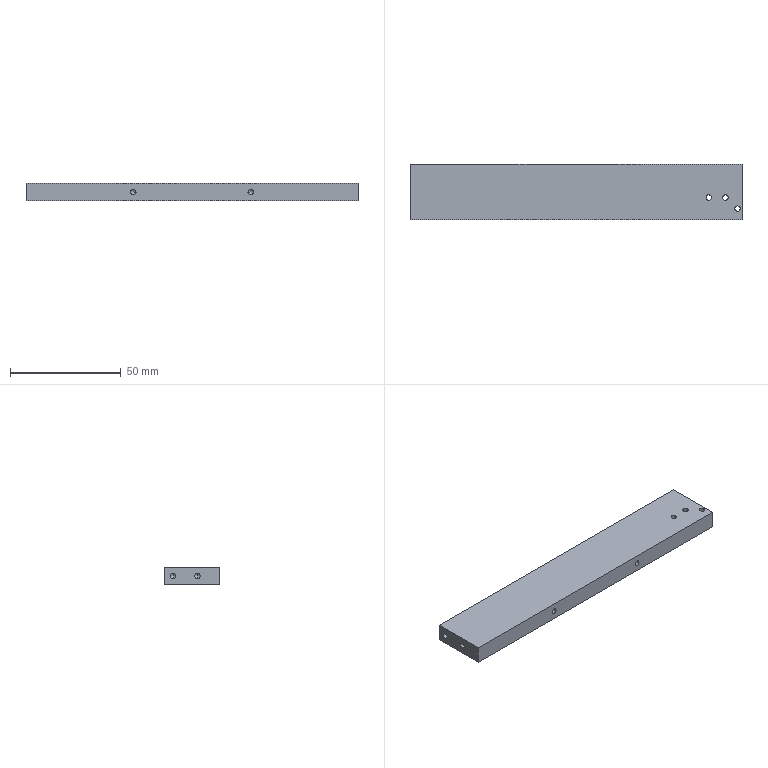Part | SolidWorks | features BaseBody 1 | 1 solid | 40 faces | box 150 x 25 x 8 mm | volume 29604 mm3 | cylinder 22 | cone 12 | plane 6 | commonest cylinder face diameters 2.459 x22
STEP:
#1=CARTESIAN_POINT('',(104.096,10.,0.));
#2=VERTEX_POINT('',#1);
#3=CARTESIAN_POINT('',(101.637,10.,0.));
#4=VERTEX_POINT('',#3);
#5=CARTESIAN_POINT('',(102.866,10.,0.));
#6=DIRECTION('',(0.,0.,-1.));
#7=DIRECTION('',(1.,0.,0.));
#8=AXIS2_PLACEMENT_3D('',#5,#6,#7);
#9=CIRCLE('',#8,1.229);
#10=EDGE_CURVE('',#2,#4,#9,.T.);
#11=ORIENTED_EDGE('',*,*,#10,.T.);
#12=CARTESIAN_POINT('',(101.637,10.,2.77));
#13=VERTEX_POINT('',#12);
#14=CARTESIAN_POINT('',(101.637,10.,-150.193));
#15=DIRECTION('',(0.,0.,1.));
#16=VECTOR('',#15,1000.);
#17=LINE('',#14,#16);
#18=EDGE_CURVE('',#4,#13,#17,.T.);
#19=ORIENTED_EDGE('',*,*,#18,.T.);
#20=CARTESIAN_POINT('',(102.866,8.771,4.));
#21=VERTEX_POINT('',#20);
#22=CARTESIAN_POINT('',(102.866,8.771,4.));
#23=CARTESIAN_POINT('',(102.146,8.771,3.28));
#24=CARTESIAN_POINT('',(101.637,9.28,2.771));
#25=CARTESIAN_POINT('',(101.637,10.,2.77));
#26=(BOUNDED_CURVE()B_SPLINE_CURVE(3,(#22,#23,#24,#25),.UNSPECIFIED.,.F.,.T.)B_SPLINE_CURVE_WITH_KNOTS((4,4),(1.571,3.142),.UNSPECIFIED.)CURVE()GEOMETRIC_REPRESENTATION_ITEM()RATIONAL_B_SPLINE_CURVE((1.,0.8047,0.8047,1.))REPRESENTATION_ITEM(''));
#27=EDGE_CURVE('',#21,#13,#26,.T.);
#28=ORIENTED_EDGE('',*,*,#27,.F.);
#29=CARTESIAN_POINT('',(104.096,10.,2.77));
#30=VERTEX_POINT('',#29);
#31=CARTESIAN_POINT('',(104.096,10.,2.77));
#32=CARTESIAN_POINT('',(104.096,9.28,2.771));
#33=CARTESIAN_POINT('',(103.587,8.771,3.28));
#34=CARTESIAN_POINT('',(102.866,8.771,4.));
#35=(BOUNDED_CURVE()B_SPLINE_CURVE(3,(#31,#32,#33,#34),.UNSPECIFIED.,.F.,.T.)B_SPLINE_CURVE_WITH_KNOTS((4,4),(0.,1.571),.UNSPECIFIED.)CURVE()GEOMETRIC_REPRESENTATION_ITEM()RATIONAL_B_SPLINE_CURVE((1.,0.8047,0.8047,1.))REPRESENTATION_ITEM(''));
#36=EDGE_CURVE('',#30,#21,#35,.T.);
#37=ORIENTED_EDGE('',*,*,#36,.F.);
#38=CARTESIAN_POINT('',(104.096,10.,-150.193));
#39=DIRECTION('',(0.,0.,1.));
#40=VECTOR('',#39,1000.);
#41=LINE('',#38,#40);
#42=EDGE_CURVE('',#2,#30,#41,.T.);
#43=ORIENTED_EDGE('',*,*,#42,.F.);
#44=EDGE_LOOP('',(#11,#19,#28,#37,#43));
#45=FACE_OUTER_BOUND('',#44,.T.);
#46=CARTESIAN_POINT('',(102.866,10.,-150.193));
#47=DIRECTION('',(0.,0.,1.));
#48=DIRECTION('',(1.,0.,0.));
#49=AXIS2_PLACEMENT_3D('',#46,#47,#48);
#50=CYLINDRICAL_SURFACE('',#49,1.229);
#51=ADVANCED_FACE('',(#45),#50,.F.);
#52=CARTESIAN_POINT('',(96.596,10.,0.));
#53=VERTEX_POINT('',#52);
#54=CARTESIAN_POINT('',(94.137,10.,0.));
#55=VERTEX_POINT('',#54);
#56=CARTESIAN_POINT('',(95.366,10.,0.));
#57=DIRECTION('',(0.,0.,-1.));
#58=DIRECTION('',(1.,0.,0.));
#59=AXIS2_PLACEMENT_3D('',#56,#57,#58);
#60=CIRCLE('',#59,1.229);
#61=EDGE_CURVE('',#53,#55,#60,.T.);
#62=ORIENTED_EDGE('',*,*,#61,.T.);
#63=CARTESIAN_POINT('',(94.137,10.,8.));
#64=VERTEX_POINT('',#63);
#65=CARTESIAN_POINT('',(94.137,10.,-150.193));
#66=DIRECTION('',(0.,0.,1.));
#67=VECTOR('',#66,1000.);
#68=LINE('',#65,#67);
#69=EDGE_CURVE('',#55,#64,#68,.T.);
#70=ORIENTED_EDGE('',*,*,#69,.T.);
#71=CARTESIAN_POINT('',(96.596,10.,8.));
#72=VERTEX_POINT('',#71);
#73=CARTESIAN_POINT('',(95.366,10.,8.));
#74=DIRECTION('',(0.,0.,-1.));
#75=DIRECTION('',(1.,0.,0.));
#76=AXIS2_PLACEMENT_3D('',#73,#74,#75);
#77=CIRCLE('',#76,1.229);
#78=EDGE_CURVE('',#72,#64,#77,.T.);
#79=ORIENTED_EDGE('',*,*,#78,.F.);
#80=CARTESIAN_POINT('',(96.596,10.,-150.193));
#81=DIRECTION('',(0.,0.,1.));
#82=VECTOR('',#81,1000.);
#83=LINE('',#80,#82);
#84=EDGE_CURVE('',#53,#72,#83,.T.);
#85=ORIENTED_EDGE('',*,*,#84,.F.);
#86=EDGE_LOOP('',(#62,#70,#79,#85));
#87=FACE_OUTER_BOUND('',#86,.T.);
#88=CARTESIAN_POINT('',(95.366,10.,-150.193));
#89=DIRECTION('',(0.,0.,1.));
#90=DIRECTION('',(1.,0.,0.));
#91=AXIS2_PLACEMENT_3D('',#88,#89,#90);
#92=CYLINDRICAL_SURFACE('',#91,1.229);
#93=ADVANCED_FACE('',(#87),#92,.F.);
#94=CARTESIAN_POINT('',(109.596,5.,0.));
#95=VERTEX_POINT('',#94);
#96=CARTESIAN_POINT('',(107.137,5.,0.));
#97=VERTEX_POINT('',#96);
#98=CARTESIAN_POINT('',(108.366,5.,0.));
#99=DIRECTION('',(0.,0.,-1.));
#100=DIRECTION('',(1.,0.,0.));
#101=AXIS2_PLACEMENT_3D('',#98,#99,#100);
#102=CIRCLE('',#101,1.229);
#103=EDGE_CURVE('',#95,#97,#102,.T.);
#104=ORIENTED_EDGE('',*,*,#103,.T.);
#105=CARTESIAN_POINT('',(107.137,5.,8.));
#106=VERTEX_POINT('',#105);
#107=CARTESIAN_POINT('',(107.137,5.,-150.193));
#108=DIRECTION('',(0.,0.,1.));
#109=VECTOR('',#108,1000.);
#110=LINE('',#107,#109);
#111=EDGE_CURVE('',#97,#106,#110,.T.);
#112=ORIENTED_EDGE('',*,*,#111,.T.);
#113=CARTESIAN_POINT('',(109.596,5.,8.));
#114=VERTEX_POINT('',#113);
#115=CARTESIAN_POINT('',(108.366,5.,8.));
#116=DIRECTION('',(0.,0.,-1.));
#117=DIRECTION('',(1.,0.,0.));
#118=AXIS2_PLACEMENT_3D('',#115,#116,#117);
#119=CIRCLE('',#118,1.229);
#120=EDGE_CURVE('',#114,#106,#119,.T.);
#121=ORIENTED_EDGE('',*,*,#120,.F.);
#122=CARTESIAN_POINT('',(109.596,5.,-150.193));
#123=DIRECTION('',(0.,0.,1.));
#124=VECTOR('',#123,1000.);
#125=LINE('',#122,#124);
#126=EDGE_CURVE('',#95,#114,#125,.T.);
#127=ORIENTED_EDGE('',*,*,#126,.F.);
#128=EDGE_LOOP('',(#104,#112,#121,#127));
#129=FACE_OUTER_BOUND('',#128,.T.);
#130=CARTESIAN_POINT('',(108.366,5.,-150.193));
#131=DIRECTION('',(0.,0.,1.));
#132=DIRECTION('',(1.,0.,0.));
#133=AXIS2_PLACEMENT_3D('',#130,#131,#132);
#134=CYLINDRICAL_SURFACE('',#133,1.229);
#135=ADVANCED_FACE('',(#129),#134,.F.);
#136=CARTESIAN_POINT('',(100.366,10.,5.229));
#137=VERTEX_POINT('',#136);
#138=CARTESIAN_POINT('',(100.366,10.,2.771));
#139=VERTEX_POINT('',#138);
#140=CARTESIAN_POINT('',(100.366,10.,4.));
#141=DIRECTION('',(1.,0.,0.));
#142=DIRECTION('',(0.,0.,-1.));
#143=AXIS2_PLACEMENT_3D('',#140,#141,#142);
#144=CIRCLE('',#143,1.23);
#145=EDGE_CURVE('',#137,#139,#144,.T.);
#146=ORIENTED_EDGE('',*,*,#145,.F.);
#147=CARTESIAN_POINT('',(101.637,10.,5.229));
#148=VERTEX_POINT('',#147);
#149=CARTESIAN_POINT('',(105.366,10.,5.229));
#150=DIRECTION('',(1.,0.,0.));
#151=VECTOR('',#150,1000.);
#152=LINE('',#149,#151);
#153=EDGE_CURVE('',#137,#148,#152,.T.);
#154=ORIENTED_EDGE('',*,*,#153,.T.);
#155=CARTESIAN_POINT('',(102.866,8.771,4.));
#156=CARTESIAN_POINT('',(102.146,8.771,4.72));
#157=CARTESIAN_POINT('',(101.637,9.28,5.23));
#158=CARTESIAN_POINT('',(101.637,10.,5.229));
#159=(BOUNDED_CURVE()B_SPLINE_CURVE(3,(#155,#156,#157,#158),.UNSPECIFIED.,.F.,.T.)B_SPLINE_CURVE_WITH_KNOTS((4,4),(4.712,6.283),.UNSPECIFIED.)CURVE()GEOMETRIC_REPRESENTATION_ITEM()RATIONAL_B_SPLINE_CURVE((1.,0.8047,0.8047,1.))REPRESENTATION_ITEM(''));
#160=EDGE_CURVE('',#21,#148,#159,.T.);
#161=ORIENTED_EDGE('',*,*,#160,.F.);
#162=ORIENTED_EDGE('',*,*,#27,.T.);
#163=CARTESIAN_POINT('',(105.366,10.,2.77));
#164=DIRECTION('',(1.,0.,0.));
#165=VECTOR('',#164,1000.);
#166=LINE('',#163,#165);
#167=EDGE_CURVE('',#139,#13,#166,.T.);
#168=ORIENTED_EDGE('',*,*,#167,.F.);
#169=EDGE_LOOP('',(#146,#154,#161,#162,#168));
#170=FACE_OUTER_BOUND('',#169,.T.);
#171=CARTESIAN_POINT('',(105.366,10.,4.));
#172=DIRECTION('',(1.,0.,0.));
#173=DIRECTION('',(0.,0.,-1.));
#174=AXIS2_PLACEMENT_3D('',#171,#172,#173);
#175=CYLINDRICAL_SURFACE('',#174,1.23);
#176=ADVANCED_FACE('',(#170),#175,.F.);
#177=CARTESIAN_POINT('',(104.096,10.,5.229));
#178=VERTEX_POINT('',#177);
#179=CARTESIAN_POINT('',(104.096,10.,5.229));
#180=CARTESIAN_POINT('',(104.096,9.28,5.23));
#181=CARTESIAN_POINT('',(103.587,8.771,4.72));
#182=CARTESIAN_POINT('',(102.866,8.771,4.));
#183=(BOUNDED_CURVE()B_SPLINE_CURVE(3,(#179,#180,#181,#182),.UNSPECIFIED.,.F.,.F.)B_SPLINE_CURVE_WITH_KNOTS((4,4),(0.,1.571),.UNSPECIFIED.)CURVE()GEOMETRIC_REPRESENTATION_ITEM()RATIONAL_B_SPLINE_CURVE((1.,0.8047,0.8047,1.))REPRESENTATION_ITEM(''));
#184=EDGE_CURVE('',#178,#21,#183,.T.);
#185=ORIENTED_EDGE('',*,*,#184,.F.);
#186=CARTESIAN_POINT('',(110.366,10.,5.23));
#187=VERTEX_POINT('',#186);
#188=CARTESIAN_POINT('',(105.366,10.,5.229));
#189=DIRECTION('',(1.,0.,0.));
#190=VECTOR('',#189,1000.);
#191=LINE('',#188,#190);
#192=EDGE_CURVE('',#178,#187,#191,.T.);
#193=ORIENTED_EDGE('',*,*,#192,.T.);
#194=CARTESIAN_POINT('',(110.366,10.,2.77));
#195=VERTEX_POINT('',#194);
#196=CARTESIAN_POINT('',(110.366,10.,4.));
#197=DIRECTION('',(-1.,0.,0.));
#198=DIRECTION('',(0.,0.,-1.));
#199=AXIS2_PLACEMENT_3D('',#196,#197,#198);
#200=CIRCLE('',#199,1.23);
#201=EDGE_CURVE('',#195,#187,#200,.T.);
#202=ORIENTED_EDGE('',*,*,#201,.F.);
#203=CARTESIAN_POINT('',(105.366,10.,2.77));
#204=DIRECTION('',(1.,0.,0.));
#205=VECTOR('',#204,1000.);
#206=LINE('',#203,#205);
#207=EDGE_CURVE('',#30,#195,#206,.T.);
#208=ORIENTED_EDGE('',*,*,#207,.F.);
#209=ORIENTED_EDGE('',*,*,#36,.T.);
#210=EDGE_LOOP('',(#185,#193,#202,#208,#209));
#211=FACE_OUTER_BOUND('',#210,.T.);
#212=CARTESIAN_POINT('',(105.366,10.,4.));
#213=DIRECTION('',(1.,0.,0.));
#214=DIRECTION('',(0.,0.,-1.));
#215=AXIS2_PLACEMENT_3D('',#212,#213,#214);
#216=CYLINDRICAL_SURFACE('',#215,1.23);
#217=ADVANCED_FACE('',(#211),#216,.F.);
#218=CARTESIAN_POINT('',(100.366,21.,5.229));
#219=VERTEX_POINT('',#218);
#220=CARTESIAN_POINT('',(100.366,21.,2.771));
#221=VERTEX_POINT('',#220);
#222=CARTESIAN_POINT('',(100.366,21.,4.));
#223=DIRECTION('',(1.,0.,0.));
#224=DIRECTION('',(0.,0.,-1.));
#225=AXIS2_PLACEMENT_3D('',#222,#223,#224);
#226=CIRCLE('',#225,1.23);
#227=EDGE_CURVE('',#219,#221,#226,.T.);
#228=ORIENTED_EDGE('',*,*,#227,.F.);
#229=CARTESIAN_POINT('',(110.366,21.,5.23));
#230=VERTEX_POINT('',#229);
#231=CARTESIAN_POINT('',(105.366,21.,5.229));
#232=DIRECTION('',(1.,0.,0.));
#233=VECTOR('',#232,1000.);
#234=LINE('',#231,#233);
#235=EDGE_CURVE('',#219,#230,#234,.T.);
#236=ORIENTED_EDGE('',*,*,#235,.T.);
#237=CARTESIAN_POINT('',(110.366,21.,2.77));
#238=VERTEX_POINT('',#237);
#239=CARTESIAN_POINT('',(110.366,21.,4.));
#240=DIRECTION('',(-1.,0.,0.));
#241=DIRECTION('',(0.,0.,-1.));
#242=AXIS2_PLACEMENT_3D('',#239,#240,#241);
#243=CIRCLE('',#242,1.23);
#244=EDGE_CURVE('',#238,#230,#243,.T.);
#245=ORIENTED_EDGE('',*,*,#244,.F.);
#246=CARTESIAN_POINT('',(105.366,21.,2.77));
#247=DIRECTION('',(1.,0.,0.));
#248=VECTOR('',#247,1000.);
#249=LINE('',#246,#248);
#250=EDGE_CURVE('',#221,#238,#249,.T.);
#251=ORIENTED_EDGE('',*,*,#250,.F.);
#252=EDGE_LOOP('',(#228,#236,#245,#251));
#253=FACE_OUTER_BOUND('',#252,.T.);
#254=CARTESIAN_POINT('',(105.366,21.,4.));
#255=DIRECTION('',(1.,0.,0.));
#256=DIRECTION('',(0.,0.,-1.));
#257=AXIS2_PLACEMENT_3D('',#254,#255,#256);
#258=CYLINDRICAL_SURFACE('',#257,1.23);
#259=ADVANCED_FACE('',(#253),#258,.F.);
#260=CARTESIAN_POINT('',(60.637,10.,4.));
#261=VERTEX_POINT('',#260);
#262=CARTESIAN_POINT('',(63.096,10.,4.));
#263=VERTEX_POINT('',#262);
#264=CARTESIAN_POINT('',(61.866,10.,4.));
#265=DIRECTION('',(0.,-1.,0.));
#266=DIRECTION('',(1.,0.,0.));
#267=AXIS2_PLACEMENT_3D('',#264,#265,#266);
#268=CIRCLE('',#267,1.23);
#269=EDGE_CURVE('',#261,#263,#268,.T.);
#270=ORIENTED_EDGE('',*,*,#269,.F.);
#271=CARTESIAN_POINT('',(60.637,0.,4.));
#272=VERTEX_POINT('',#271);
#273=CARTESIAN_POINT('',(60.637,5.,4.));
#274=DIRECTION('',(0.,-1.,0.));
#275=VECTOR('',#274,1000.);
#276=LINE('',#273,#275);
#277=EDGE_CURVE('',#261,#272,#276,.T.);
#278=ORIENTED_EDGE('',*,*,#277,.T.);
#279=CARTESIAN_POINT('',(63.096,0.,4.));
#280=VERTEX_POINT('',#279);
#281=CARTESIAN_POINT('',(61.866,0.,4.));
#282=DIRECTION('',(0.,1.,0.));
#283=DIRECTION('',(1.,0.,0.));
#284=AXIS2_PLACEMENT_3D('',#281,#282,#283);
#285=CIRCLE('',#284,1.23);
#286=EDGE_CURVE('',#280,#272,#285,.T.);
#287=ORIENTED_EDGE('',*,*,#286,.F.);
#288=CARTESIAN_POINT('',(63.096,5.,4.));
#289=DIRECTION('',(0.,-1.,0.));
#290=VECTOR('',#289,1000.);
#291=LINE('',#288,#290);
#292=EDGE_CURVE('',#263,#280,#291,.T.);
#293=ORIENTED_EDGE('',*,*,#292,.F.);
#294=EDGE_LOOP('',(#270,#278,#287,#293));
#295=FACE_OUTER_BOUND('',#294,.T.);
#296=CARTESIAN_POINT('',(61.866,5.,4.));
#297=DIRECTION('',(0.,-1.,0.));
#298=DIRECTION('',(1.,0.,0.));
#299=AXIS2_PLACEMENT_3D('',#296,#297,#298);
#300=CYLINDRICAL_SURFACE('',#299,1.23);
#301=ADVANCED_FACE('',(#295),#300,.F.);
#302=CARTESIAN_POINT('',(7.637,10.,4.));
#303=VERTEX_POINT('',#302);
#304=CARTESIAN_POINT('',(10.096,10.,4.));
#305=VERTEX_POINT('',#304);
#306=CARTESIAN_POINT('',(8.866,10.,4.));
#307=DIRECTION('',(0.,-1.,0.));
#308=DIRECTION('',(1.,0.,0.));
#309=AXIS2_PLACEMENT_3D('',#306,#307,#308);
#310=CIRCLE('',#309,1.229);
#311=EDGE_CURVE('',#303,#305,#310,.T.);
#312=ORIENTED_EDGE('',*,*,#311,.F.);
#313=CARTESIAN_POINT('',(7.637,0.,4.));
#314=VERTEX_POINT('',#313);
#315=CARTESIAN_POINT('',(7.637,5.,4.));
#316=DIRECTION('',(0.,-1.,0.));
#317=VECTOR('',#316,1000.);
#318=LINE('',#315,#317);
#319=EDGE_CURVE('',#303,#314,#318,.T.);
#320=ORIENTED_EDGE('',*,*,#319,.T.);
#321=CARTESIAN_POINT('',(10.096,0.,4.));
#322=VERTEX_POINT('',#321);
#323=CARTESIAN_POINT('',(8.866,0.,4.));
#324=DIRECTION('',(0.,1.,0.));
#325=DIRECTION('',(1.,0.,0.));
#326=AXIS2_PLACEMENT_3D('',#323,#324,#325);
#327=CIRCLE('',#326,1.229);
#328=EDGE_CURVE('',#322,#314,#327,.T.);
#329=ORIENTED_EDGE('',*,*,#328,.F.);
#330=CARTESIAN_POINT('',(10.096,5.,4.));
#331=DIRECTION('',(0.,-1.,0.));
#332=VECTOR('',#331,1000.);
#333=LINE('',#330,#332);
#334=EDGE_CURVE('',#305,#322,#333,.T.);
#335=ORIENTED_EDGE('',*,*,#334,.F.);
#336=EDGE_LOOP('',(#312,#320,#329,#335));
#337=FACE_OUTER_BOUND('',#336,.T.);
#338=CARTESIAN_POINT('',(8.866,5.,4.));
#339=DIRECTION('',(0.,-1.,0.));
#340=DIRECTION('',(1.,0.,0.));
#341=AXIS2_PLACEMENT_3D('',#338,#339,#340);
#342=CYLINDRICAL_SURFACE('',#341,1.229);
#343=ADVANCED_FACE('',(#337),#342,.F.);
#344=CARTESIAN_POINT('',(-29.634,10.,2.771));
#345=VERTEX_POINT('',#344);
#346=CARTESIAN_POINT('',(-29.634,10.,5.229));
#347=VERTEX_POINT('',#346);
#348=CARTESIAN_POINT('',(-29.634,10.,4.));
#349=DIRECTION('',(-1.,0.,0.));
#350=DIRECTION('',(0.,0.,1.));
#351=AXIS2_PLACEMENT_3D('',#348,#349,#350);
#352=CIRCLE('',#351,1.229);
#353=EDGE_CURVE('',#345,#347,#352,.T.);
#354=ORIENTED_EDGE('',*,*,#353,.F.);
#355=CARTESIAN_POINT('',(-39.634,10.,2.77));
#356=VERTEX_POINT('',#355);
#357=CARTESIAN_POINT('',(-34.634,10.,2.77));
#358=DIRECTION('',(-1.,0.,0.));
#359=VECTOR('',#358,1000.);
#360=LINE('',#357,#359);
#361=EDGE_CURVE('',#345,#356,#360,.T.);
#362=ORIENTED_EDGE('',*,*,#361,.T.);
#363=CARTESIAN_POINT('',(-39.634,10.,5.229));
#364=VERTEX_POINT('',#363);
#365=CARTESIAN_POINT('',(-39.634,10.,4.));
#366=DIRECTION('',(1.,0.,0.));
#367=DIRECTION('',(0.,0.,1.));
#368=AXIS2_PLACEMENT_3D('',#365,#366,#367);
#369=CIRCLE('',#368,1.229);
#370=EDGE_CURVE('',#364,#356,#369,.T.);
#371=ORIENTED_EDGE('',*,*,#370,.F.);
#372=CARTESIAN_POINT('',(-34.634,10.,5.229));
#373=DIRECTION('',(-1.,0.,0.));
#374=VECTOR('',#373,1000.);
#375=LINE('',#372,#374);
#376=EDGE_CURVE('',#347,#364,#375,.T.);
#377=ORIENTED_EDGE('',*,*,#376,.F.);
#378=EDGE_LOOP('',(#354,#362,#371,#377));
#379=FACE_OUTER_BOUND('',#378,.T.);
#380=CARTESIAN_POINT('',(-34.634,10.,4.));
#381=DIRECTION('',(-1.,0.,0.));
#382=DIRECTION('',(0.,0.,1.));
#383=AXIS2_PLACEMENT_3D('',#380,#381,#382);
#384=CYLINDRICAL_SURFACE('',#383,1.229);
#385=ADVANCED_FACE('',(#379),#384,.F.);
#386=CARTESIAN_POINT('',(-29.634,21.,2.771));
#387=VERTEX_POINT('',#386);
#388=CARTESIAN_POINT('',(-29.634,21.,5.229));
#389=VERTEX_POINT('',#388);
#390=CARTESIAN_POINT('',(-29.634,21.,4.));
#391=DIRECTION('',(-1.,0.,0.));
#392=DIRECTION('',(0.,0.,1.));
#393=AXIS2_PLACEMENT_3D('',#390,#391,#392);
#394=CIRCLE('',#393,1.229);
#395=EDGE_CURVE('',#387,#389,#394,.T.);
#396=ORIENTED_EDGE('',*,*,#395,.F.);
#397=CARTESIAN_POINT('',(-39.634,21.,2.77));
#398=VERTEX_POINT('',#397);
#399=CARTESIAN_POINT('',(-34.634,21.,2.77));
#400=DIRECTION('',(-1.,0.,0.));
#401=VECTOR('',#400,1000.);
#402=LINE('',#399,#401);
#403=EDGE_CURVE('',#387,#398,#402,.T.);
#404=ORIENTED_EDGE('',*,*,#403,.T.);
#405=CARTESIAN_POINT('',(-39.634,21.,5.229));
#406=VERTEX_POINT('',#405);
#407=CARTESIAN_POINT('',(-39.634,21.,4.));
#408=DIRECTION('',(1.,0.,0.));
#409=DIRECTION('',(0.,0.,1.));
#410=AXIS2_PLACEMENT_3D('',#407,#408,#409);
#411=CIRCLE('',#410,1.229);
#412=EDGE_CURVE('',#406,#398,#411,.T.);
#413=ORIENTED_EDGE('',*,*,#412,.F.);
#414=CARTESIAN_POINT('',(-34.634,21.,5.229));
#415=DIRECTION('',(-1.,0.,0.));
#416=VECTOR('',#415,1000.);
#417=LINE('',#414,#416);
#418=EDGE_CURVE('',#389,#406,#417,.T.);
#419=ORIENTED_EDGE('',*,*,#418,.F.);
#420=EDGE_LOOP('',(#396,#404,#413,#419));
#421=FACE_OUTER_BOUND('',#420,.T.);
#422=CARTESIAN_POINT('',(-34.634,21.,4.));
#423=DIRECTION('',(-1.,0.,0.));
#424=DIRECTION('',(0.,0.,1.));
#425=AXIS2_PLACEMENT_3D('',#422,#423,#424);
#426=CYLINDRICAL_SURFACE('',#425,1.229);
#427=ADVANCED_FACE('',(#421),#426,.F.);
#428=CARTESIAN_POINT('',(99.628,10.,4.));
#429=VERTEX_POINT('',#428);
#430=CARTESIAN_POINT('',(100.366,10.,2.771));
#431=DIRECTION('',(0.515,0.,-0.8572));
#432=VECTOR('',#431,1000.);
#433=LINE('',#430,#432);
#434=EDGE_CURVE('',#429,#139,#433,.T.);
#435=ORIENTED_EDGE('',*,*,#434,.F.);
#436=CARTESIAN_POINT('',(100.366,10.,5.229));
#437=DIRECTION('',(0.515,0.,0.8572));
#438=VECTOR('',#437,1000.);
#439=LINE('',#436,#438);
#440=EDGE_CURVE('',#429,#137,#439,.T.);
#441=ORIENTED_EDGE('',*,*,#440,.T.);
#442=ORIENTED_EDGE('',*,*,#145,.T.);
#443=EDGE_LOOP('',(#435,#441,#442));
#444=FACE_OUTER_BOUND('',#443,.T.);
#445=CARTESIAN_POINT('',(100.366,10.,4.));
#446=DIRECTION('',(1.,0.,0.));
#447=DIRECTION('',(0.,0.,-1.));
#448=AXIS2_PLACEMENT_3D('',#445,#446,#447);
#449=CONICAL_SURFACE('',#448,1.229,1.03);
#450=ADVANCED_FACE('',(#444),#449,.F.);
#451=ORIENTED_EDGE('',*,*,#160,.T.);
#452=CARTESIAN_POINT('',(101.637,10.,8.));
#453=VERTEX_POINT('',#452);
#454=CARTESIAN_POINT('',(101.637,10.,-150.193));
#455=DIRECTION('',(0.,0.,1.));
#456=VECTOR('',#455,1000.);
#457=LINE('',#454,#456);
#458=EDGE_CURVE('',#148,#453,#457,.T.);
#459=ORIENTED_EDGE('',*,*,#458,.T.);
#460=CARTESIAN_POINT('',(104.096,10.,8.));
#461=VERTEX_POINT('',#460);
#462=CARTESIAN_POINT('',(102.866,10.,8.));
#463=DIRECTION('',(0.,0.,-1.));
#464=DIRECTION('',(1.,0.,0.));
#465=AXIS2_PLACEMENT_3D('',#462,#463,#464);
#466=CIRCLE('',#465,1.229);
#467=EDGE_CURVE('',#461,#453,#466,.T.);
#468=ORIENTED_EDGE('',*,*,#467,.F.);
#469=CARTESIAN_POINT('',(104.096,10.,-150.193));
#470=DIRECTION('',(0.,0.,1.));
#471=VECTOR('',#470,1000.);
#472=LINE('',#469,#471);
#473=EDGE_CURVE('',#178,#461,#472,.T.);
#474=ORIENTED_EDGE('',*,*,#473,.F.);
#475=ORIENTED_EDGE('',*,*,#184,.T.);
#476=EDGE_LOOP('',(#451,#459,#468,#474,#475));
#477=FACE_OUTER_BOUND('',#476,.T.);
#478=CARTESIAN_POINT('',(102.866,10.,-150.193));
#479=DIRECTION('',(0.,0.,1.));
#480=DIRECTION('',(1.,0.,0.));
#481=AXIS2_PLACEMENT_3D('',#478,#479,#480);
#482=CYLINDRICAL_SURFACE('',#481,1.229);
#483=ADVANCED_FACE('',(#477),#482,.F.);
#484=CARTESIAN_POINT('',(99.628,21.,4.));
#485=VERTEX_POINT('',#484);
#486=CARTESIAN_POINT('',(100.366,21.,2.771));
#487=DIRECTION('',(0.515,0.,-0.8572));
#488=VECTOR('',#487,1000.);
#489=LINE('',#486,#488);
#490=EDGE_CURVE('',#485,#221,#489,.T.);
#491=ORIENTED_EDGE('',*,*,#490,.F.);
#492=CARTESIAN_POINT('',(100.366,21.,5.229));
#493=DIRECTION('',(0.515,0.,0.8572));
#494=VECTOR('',#493,1000.);
#495=LINE('',#492,#494);
#496=EDGE_CURVE('',#485,#219,#495,.T.);
#497=ORIENTED_EDGE('',*,*,#496,.T.);
#498=ORIENTED_EDGE('',*,*,#227,.T.);
#499=EDGE_LOOP('',(#491,#497,#498));
#500=FACE_OUTER_BOUND('',#499,.T.);
#501=CARTESIAN_POINT('',(100.366,21.,4.));
#502=DIRECTION('',(1.,0.,0.));
#503=DIRECTION('',(0.,0.,-1.));
#504=AXIS2_PLACEMENT_3D('',#501,#502,#503);
#505=CONICAL_SURFACE('',#504,1.229,1.03);
#506=ADVANCED_FACE('',(#500),#505,.F.);
#507=CARTESIAN_POINT('',(61.866,10.739,4.));
#508=VERTEX_POINT('',#507);
#509=CARTESIAN_POINT('',(63.096,10.,4.));
#510=DIRECTION('',(0.8572,-0.515,0.));
#511=VECTOR('',#510,1000.);
#512=LINE('',#509,#511);
#513=EDGE_CURVE('',#508,#263,#512,.T.);
#514=ORIENTED_EDGE('',*,*,#513,.F.);
#515=CARTESIAN_POINT('',(60.637,10.,4.));
#516=DIRECTION('',(-0.8572,-0.515,0.));
#517=VECTOR('',#516,1000.);
#518=LINE('',#515,#517);
#519=EDGE_CURVE('',#508,#261,#518,.T.);
#520=ORIENTED_EDGE('',*,*,#519,.T.);
#521=ORIENTED_EDGE('',*,*,#269,.T.);
#522=EDGE_LOOP('',(#514,#520,#521));
#523=FACE_OUTER_BOUND('',#522,.T.);
#524=CARTESIAN_POINT('',(61.866,10.,4.));
#525=DIRECTION('',(0.,-1.,0.));
#526=DIRECTION('',(1.,0.,0.));
#527=AXIS2_PLACEMENT_3D('',#524,#525,#526);
#528=CONICAL_SURFACE('',#527,1.229,1.03);
#529=ADVANCED_FACE('',(#523),#528,.F.);
#530=CARTESIAN_POINT('',(8.866,10.739,4.));
#531=VERTEX_POINT('',#530);
#532=CARTESIAN_POINT('',(10.096,10.,4.));
#533=DIRECTION('',(0.8572,-0.515,0.));
#534=VECTOR('',#533,1000.);
#535=LINE('',#532,#534);
#536=EDGE_CURVE('',#531,#305,#535,.T.);
#537=ORIENTED_EDGE('',*,*,#536,.F.);
#538=CARTESIAN_POINT('',(7.637,10.,4.));
#539=DIRECTION('',(-0.8572,-0.515,0.));
#540=VECTOR('',#539,1000.);
#541=LINE('',#538,#540);
#542=EDGE_CURVE('',#531,#303,#541,.T.);
#543=ORIENTED_EDGE('',*,*,#542,.T.);
#544=ORIENTED_EDGE('',*,*,#311,.T.);
#545=EDGE_LOOP('',(#537,#543,#544));
#546=FACE_OUTER_BOUND('',#545,.T.);
#547=CARTESIAN_POINT('',(8.866,10.,4.));
#548=DIRECTION('',(0.,-1.,0.));
#549=DIRECTION('',(1.,0.,0.));
#550=AXIS2_PLACEMENT_3D('',#547,#548,#549);
#551=CONICAL_SURFACE('',#550,1.229,1.03);
#552=ADVANCED_FACE('',(#546),#551,.F.);
#553=CARTESIAN_POINT('',(-28.895,10.,4.));
#554=VERTEX_POINT('',#553);
#555=CARTESIAN_POINT('',(-29.634,10.,5.229));
#556=DIRECTION('',(-0.515,0.,0.8572));
#557=VECTOR('',#556,1000.);
#558=LINE('',#555,#557);
#559=EDGE_CURVE('',#554,#347,#558,.T.);
#560=ORIENTED_EDGE('',*,*,#559,.F.);
#561=CARTESIAN_POINT('',(-29.634,10.,2.771));
#562=DIRECTION('',(-0.515,0.,-0.8572));
#563=VECTOR('',#562,1000.);
#564=LINE('',#561,#563);
#565=EDGE_CURVE('',#554,#345,#564,.T.);
#566=ORIENTED_EDGE('',*,*,#565,.T.);
#567=ORIENTED_EDGE('',*,*,#353,.T.);
#568=EDGE_LOOP('',(#560,#566,#567));
#569=FACE_OUTER_BOUND('',#568,.T.);
#570=CARTESIAN_POINT('',(-29.634,10.,4.));
#571=DIRECTION('',(-1.,0.,0.));
#572=DIRECTION('',(0.,0.,1.));
#573=AXIS2_PLACEMENT_3D('',#570,#571,#572);
#574=CONICAL_SURFACE('',#573,1.229,1.03);
#575=ADVANCED_FACE('',(#569),#574,.F.);
#576=CARTESIAN_POINT('',(-28.895,21.,4.));
#577=VERTEX_POINT('',#576);
#578=CARTESIAN_POINT('',(-29.634,21.,5.229));
#579=DIRECTION('',(-0.515,0.,0.8572));
#580=VECTOR('',#579,1000.);
#581=LINE('',#578,#580);
#582=EDGE_CURVE('',#577,#389,#581,.T.);
#583=ORIENTED_EDGE('',*,*,#582,.F.);
#584=CARTESIAN_POINT('',(-29.634,21.,2.771));
#585=DIRECTION('',(-0.515,0.,-0.8572));
#586=VECTOR('',#585,1000.);
#587=LINE('',#584,#586);
#588=EDGE_CURVE('',#577,#387,#587,.T.);
#589=ORIENTED_EDGE('',*,*,#588,.T.);
#590=ORIENTED_EDGE('',*,*,#395,.T.);
#591=EDGE_LOOP('',(#583,#589,#590));
#592=FACE_OUTER_BOUND('',#591,.T.);
#593=CARTESIAN_POINT('',(-29.634,21.,4.));
#594=DIRECTION('',(-1.,0.,0.));
#595=DIRECTION('',(0.,0.,1.));
#596=AXIS2_PLACEMENT_3D('',#593,#594,#595);
#597=CONICAL_SURFACE('',#596,1.229,1.03);
#598=ADVANCED_FACE('',(#592),#597,.F.);
#599=ORIENTED_EDGE('',*,*,#10,.F.);
#600=CARTESIAN_POINT('',(102.866,10.,0.));
#601=DIRECTION('',(0.,0.,-1.));
#602=DIRECTION('',(1.,0.,0.));
#603=AXIS2_PLACEMENT_3D('',#600,#601,#602);
#604=CIRCLE('',#603,1.229);
#605=EDGE_CURVE('',#4,#2,#604,.T.);
#606=ORIENTED_EDGE('',*,*,#605,.F.);
#607=EDGE_LOOP('',(#599,#606));
#608=FACE_BOUND('',#607,.T.);
#609=ORIENTED_EDGE('',*,*,#61,.F.);
#610=CARTESIAN_POINT('',(95.366,10.,0.));
#611=DIRECTION('',(0.,0.,-1.));
#612=DIRECTION('',(1.,0.,0.));
#613=AXIS2_PLACEMENT_3D('',#610,#611,#612);
#614=CIRCLE('',#613,1.229);
#615=EDGE_CURVE('',#55,#53,#614,.T.);
#616=ORIENTED_EDGE('',*,*,#615,.F.);
#617=EDGE_LOOP('',(#609,#616));
#618=FACE_BOUND('',#617,.T.);
#619=ORIENTED_EDGE('',*,*,#103,.F.);
#620=CARTESIAN_POINT('',(108.366,5.,0.));
#621=DIRECTION('',(0.,0.,-1.));
#622=DIRECTION('',(1.,0.,0.));
#623=AXIS2_PLACEMENT_3D('',#620,#621,#622);
#624=CIRCLE('',#623,1.229);
#625=EDGE_CURVE('',#97,#95,#624,.T.);
#626=ORIENTED_EDGE('',*,*,#625,.F.);
#627=EDGE_LOOP('',(#619,#626));
#628=FACE_BOUND('',#627,.T.);
#629=CARTESIAN_POINT('',(110.366,0.,0.));
#630=VERTEX_POINT('',#629);
#631=CARTESIAN_POINT('',(110.366,25.,0.));
#632=VERTEX_POINT('',#631);
#633=CARTESIAN_POINT('',(110.366,12.5,0.));
#634=DIRECTION('',(0.,1.,0.));
#635=VECTOR('',#634,1000.);
#636=LINE('',#633,#635);
#637=EDGE_CURVE('',#630,#632,#636,.T.);
#638=ORIENTED_EDGE('',*,*,#637,.F.);
#639=CARTESIAN_POINT('',(-39.634,0.,0.));
#640=VERTEX_POINT('',#639);
#641=CARTESIAN_POINT('',(35.366,0.,0.));
#642=DIRECTION('',(1.,0.,0.));
#643=VECTOR('',#642,1000.);
#644=LINE('',#641,#643);
#645=EDGE_CURVE('',#640,#630,#644,.T.);
#646=ORIENTED_EDGE('',*,*,#645,.F.);
#647=CARTESIAN_POINT('',(-39.634,25.,0.));
#648=VERTEX_POINT('',#647);
#649=CARTESIAN_POINT('',(-39.634,12.5,0.));
#650=DIRECTION('',(0.,-1.,0.));
#651=VECTOR('',#650,1000.);
#652=LINE('',#649,#651);
#653=EDGE_CURVE('',#648,#640,#652,.T.);
#654=ORIENTED_EDGE('',*,*,#653,.F.);
#655=CARTESIAN_POINT('',(35.366,25.,0.));
#656=DIRECTION('',(-1.,0.,0.));
#657=VECTOR('',#656,1000.);
#658=LINE('',#655,#657);
#659=EDGE_CURVE('',#632,#648,#658,.T.);
#660=ORIENTED_EDGE('',*,*,#659,.F.);
#661=EDGE_LOOP('',(#638,#646,#654,#660));
#662=FACE_OUTER_BOUND('',#661,.T.);
#663=CARTESIAN_POINT('',(35.366,12.5,0.));
#664=DIRECTION('',(0.,0.,1.));
#665=DIRECTION('',(1.,0.,0.));
#666=AXIS2_PLACEMENT_3D('',#663,#664,#665);
#667=PLANE('',#666);
#668=ADVANCED_FACE('',(#608,#618,#628,#662),#667,.F.);
#669=ORIENTED_EDGE('',*,*,#18,.F.);
#670=ORIENTED_EDGE('',*,*,#605,.T.);
#671=ORIENTED_EDGE('',*,*,#42,.T.);
#672=CARTESIAN_POINT('',(102.866,11.23,4.));
#673=VERTEX_POINT('',#672);
#674=CARTESIAN_POINT('',(102.866,11.23,4.));
#675=CARTESIAN_POINT('',(103.587,11.23,3.28));
#676=CARTESIAN_POINT('',(104.096,10.72,2.771));
#677=CARTESIAN_POINT('',(104.096,10.,2.77));
#678=(BOUNDED_CURVE()B_SPLINE_CURVE(3,(#674,#675,#676,#677),.UNSPECIFIED.,.F.,.F.)B_SPLINE_CURVE_WITH_KNOTS((4,4),(4.712,6.283),.UNSPECIFIED.)CURVE()GEOMETRIC_REPRESENTATION_ITEM()RATIONAL_B_SPLINE_CURVE((1.,0.8047,0.8047,1.))REPRESENTATION_ITEM(''));
#679=EDGE_CURVE('',#673,#30,#678,.T.);
#680=ORIENTED_EDGE('',*,*,#679,.F.);
#681=CARTESIAN_POINT('',(101.637,10.,2.77));
#682=CARTESIAN_POINT('',(101.637,10.72,2.771));
#683=CARTESIAN_POINT('',(102.146,11.23,3.28));
#684=CARTESIAN_POINT('',(102.866,11.23,4.));
#685=(BOUNDED_CURVE()B_SPLINE_CURVE(3,(#681,#682,#683,#684),.UNSPECIFIED.,.F.,.T.)B_SPLINE_CURVE_WITH_KNOTS((4,4),(3.142,4.712),.UNSPECIFIED.)CURVE()GEOMETRIC_REPRESENTATION_ITEM()RATIONAL_B_SPLINE_CURVE((1.,0.8047,0.8047,1.))REPRESENTATION_ITEM(''));
#686=EDGE_CURVE('',#13,#673,#685,.T.);
#687=ORIENTED_EDGE('',*,*,#686,.F.);
#688=EDGE_LOOP('',(#669,#670,#671,#680,#687));
#689=FACE_OUTER_BOUND('',#688,.T.);
#690=CARTESIAN_POINT('',(102.866,10.,-150.193));
#691=DIRECTION('',(0.,0.,1.));
#692=DIRECTION('',(1.,0.,0.));
#693=AXIS2_PLACEMENT_3D('',#690,#691,#692);
#694=CYLINDRICAL_SURFACE('',#693,1.229);
#695=ADVANCED_FACE('',(#689),#694,.F.);
#696=ORIENTED_EDGE('',*,*,#69,.F.);
#697=ORIENTED_EDGE('',*,*,#615,.T.);
#698=ORIENTED_EDGE('',*,*,#84,.T.);
#699=CARTESIAN_POINT('',(95.366,10.,8.));
#700=DIRECTION('',(0.,0.,-1.));
#701=DIRECTION('',(1.,0.,0.));
#702=AXIS2_PLACEMENT_3D('',#699,#700,#701);
#703=CIRCLE('',#702,1.229);
#704=EDGE_CURVE('',#64,#72,#703,.T.);
#705=ORIENTED_EDGE('',*,*,#704,.F.);
#706=EDGE_LOOP('',(#696,#697,#698,#705));
#707=FACE_OUTER_BOUND('',#706,.T.);
#708=CARTESIAN_POINT('',(95.366,10.,-150.193));
#709=DIRECTION('',(0.,0.,1.));
#710=DIRECTION('',(1.,0.,0.));
#711=AXIS2_PLACEMENT_3D('',#708,#709,#710);
#712=CYLINDRICAL_SURFACE('',#711,1.229);
#713=ADVANCED_FACE('',(#707),#712,.F.);
#714=ORIENTED_EDGE('',*,*,#111,.F.);
#715=ORIENTED_EDGE('',*,*,#625,.T.);
#716=ORIENTED_EDGE('',*,*,#126,.T.);
#717=CARTESIAN_POINT('',(108.366,5.,8.));
#718=DIRECTION('',(0.,0.,-1.));
#719=DIRECTION('',(1.,0.,0.));
#720=AXIS2_PLACEMENT_3D('',#717,#718,#719);
#721=CIRCLE('',#720,1.229);
#722=EDGE_CURVE('',#106,#114,#721,.T.);
#723=ORIENTED_EDGE('',*,*,#722,.F.);
#724=EDGE_LOOP('',(#714,#715,#716,#723));
#725=FACE_OUTER_BOUND('',#724,.T.);
#726=CARTESIAN_POINT('',(108.366,5.,-150.193));
#727=DIRECTION('',(0.,0.,1.));
#728=DIRECTION('',(1.,0.,0.));
#729=AXIS2_PLACEMENT_3D('',#726,#727,#728);
#730=CYLINDRICAL_SURFACE('',#729,1.229);
#731=ADVANCED_FACE('',(#725),#730,.F.);
#732=ORIENTED_EDGE('',*,*,#659,.T.);
#733=CARTESIAN_POINT('',(-39.634,25.,8.));
#734=VERTEX_POINT('',#733);
#735=CARTESIAN_POINT('',(-39.634,25.,0.));
#736=DIRECTION('',(0.,0.,1.));
#737=VECTOR('',#736,1000.);
#738=LINE('',#735,#737);
#739=EDGE_CURVE('',#648,#734,#738,.T.);
#740=ORIENTED_EDGE('',*,*,#739,.T.);
#741=CARTESIAN_POINT('',(110.366,25.,8.));
#742=VERTEX_POINT('',#741);
#743=CARTESIAN_POINT('',(-39.634,25.,8.));
#744=DIRECTION('',(1.,0.,0.));
#745=VECTOR('',#744,1000.);
#746=LINE('',#743,#745);
#747=EDGE_CURVE('',#734,#742,#746,.T.);
#748=ORIENTED_EDGE('',*,*,#747,.T.);
#749=CARTESIAN_POINT('',(110.366,25.,0.));
#750=DIRECTION('',(0.,0.,-1.));
#751=VECTOR('',#750,1000.);
#752=LINE('',#749,#751);
#753=EDGE_CURVE('',#742,#632,#752,.T.);
#754=ORIENTED_EDGE('',*,*,#753,.T.);
#755=EDGE_LOOP('',(#732,#740,#748,#754));
#756=FACE_OUTER_BOUND('',#755,.T.);
#757=CARTESIAN_POINT('',(-39.634,25.,0.));
#758=DIRECTION('',(0.,1.,0.));
#759=DIRECTION('',(0.,0.,1.));
#760=AXIS2_PLACEMENT_3D('',#757,#758,#759);
#761=PLANE('',#760);
#762=ADVANCED_FACE('',(#756),#761,.T.);
#763=ORIENTED_EDGE('',*,*,#201,.T.);
#764=CARTESIAN_POINT('',(110.366,10.,4.));
#765=DIRECTION('',(-1.,0.,0.));
#766=DIRECTION('',(0.,0.,-1.));
#767=AXIS2_PLACEMENT_3D('',#764,#765,#766);
#768=CIRCLE('',#767,1.23);
#769=EDGE_CURVE('',#187,#195,#768,.T.);
#770=ORIENTED_EDGE('',*,*,#769,.T.);
#771=EDGE_LOOP('',(#763,#770));
#772=FACE_BOUND('',#771,.T.);
#773=ORIENTED_EDGE('',*,*,#244,.T.);
#774=CARTESIAN_POINT('',(110.366,21.,4.));
#775=DIRECTION('',(-1.,0.,0.));
#776=DIRECTION('',(0.,0.,-1.));
#777=AXIS2_PLACEMENT_3D('',#774,#775,#776);
#778=CIRCLE('',#777,1.23);
#779=EDGE_CURVE('',#230,#238,#778,.T.);
#780=ORIENTED_EDGE('',*,*,#779,.T.);
#781=EDGE_LOOP('',(#773,#780));
#782=FACE_BOUND('',#781,.T.);
#783=ORIENTED_EDGE('',*,*,#637,.T.);
#784=ORIENTED_EDGE('',*,*,#753,.F.);
#785=CARTESIAN_POINT('',(110.366,0.,8.));
#786=VERTEX_POINT('',#785);
#787=CARTESIAN_POINT('',(110.366,25.,8.));
#788=DIRECTION('',(0.,-1.,0.));
#789=VECTOR('',#788,1000.);
#790=LINE('',#787,#789);
#791=EDGE_CURVE('',#742,#786,#790,.T.);
#792=ORIENTED_EDGE('',*,*,#791,.T.);
#793=CARTESIAN_POINT('',(110.366,0.,0.));
#794=DIRECTION('',(0.,0.,-1.));
#795=VECTOR('',#794,1000.);
#796=LINE('',#793,#795);
#797=EDGE_CURVE('',#786,#630,#796,.T.);
#798=ORIENTED_EDGE('',*,*,#797,.T.);
#799=EDGE_LOOP('',(#783,#784,#792,#798));
#800=FACE_OUTER_BOUND('',#799,.T.);
#801=CARTESIAN_POINT('',(110.366,25.,0.));
#802=DIRECTION('',(1.,0.,0.));
#803=DIRECTION('',(0.,0.,-1.));
#804=AXIS2_PLACEMENT_3D('',#801,#802,#803);
#805=PLANE('',#804);
#806=ADVANCED_FACE('',(#772,#782,#800),#805,.T.);
#807=ORIENTED_EDGE('',*,*,#286,.T.);
#808=CARTESIAN_POINT('',(61.866,0.,4.));
#809=DIRECTION('',(0.,1.,0.));
#810=DIRECTION('',(1.,0.,0.));
#811=AXIS2_PLACEMENT_3D('',#808,#809,#810);
#812=CIRCLE('',#811,1.23);
#813=EDGE_CURVE('',#272,#280,#812,.T.);
#814=ORIENTED_EDGE('',*,*,#813,.T.);
#815=EDGE_LOOP('',(#807,#814));
#816=FACE_BOUND('',#815,.T.);
#817=ORIENTED_EDGE('',*,*,#328,.T.);
#818=CARTESIAN_POINT('',(8.866,0.,4.));
#819=DIRECTION('',(0.,1.,0.));
#820=DIRECTION('',(1.,0.,0.));
#821=AXIS2_PLACEMENT_3D('',#818,#819,#820);
#822=CIRCLE('',#821,1.229);
#823=EDGE_CURVE('',#314,#322,#822,.T.);
#824=ORIENTED_EDGE('',*,*,#823,.T.);
#825=EDGE_LOOP('',(#817,#824));
#826=FACE_BOUND('',#825,.T.);
#827=ORIENTED_EDGE('',*,*,#645,.T.);
#828=ORIENTED_EDGE('',*,*,#797,.F.);
#829=CARTESIAN_POINT('',(-39.634,0.,8.));
#830=VERTEX_POINT('',#829);
#831=CARTESIAN_POINT('',(110.366,0.,8.));
#832=DIRECTION('',(-1.,0.,0.));
#833=VECTOR('',#832,1000.);
#834=LINE('',#831,#833);
#835=EDGE_CURVE('',#786,#830,#834,.T.);
#836=ORIENTED_EDGE('',*,*,#835,.T.);
#837=CARTESIAN_POINT('',(-39.634,0.,0.));
#838=DIRECTION('',(0.,0.,-1.));
#839=VECTOR('',#838,1000.);
#840=LINE('',#837,#839);
#841=EDGE_CURVE('',#830,#640,#840,.T.);
#842=ORIENTED_EDGE('',*,*,#841,.T.);
#843=EDGE_LOOP('',(#827,#828,#836,#842));
#844=FACE_OUTER_BOUND('',#843,.T.);
#845=CARTESIAN_POINT('',(110.366,0.,0.));
#846=DIRECTION('',(0.,-1.,0.));
#847=DIRECTION('',(0.,0.,-1.));
#848=AXIS2_PLACEMENT_3D('',#845,#846,#847);
#849=PLANE('',#848);
#850=ADVANCED_FACE('',(#816,#826,#844),#849,.T.);
#851=ORIENTED_EDGE('',*,*,#370,.T.);
#852=CARTESIAN_POINT('',(-39.634,10.,4.));
#853=DIRECTION('',(1.,0.,0.));
#854=DIRECTION('',(0.,0.,1.));
#855=AXIS2_PLACEMENT_3D('',#852,#853,#854);
#856=CIRCLE('',#855,1.229);
#857=EDGE_CURVE('',#356,#364,#856,.T.);
#858=ORIENTED_EDGE('',*,*,#857,.T.);
#859=EDGE_LOOP('',(#851,#858));
#860=FACE_BOUND('',#859,.T.);
#861=ORIENTED_EDGE('',*,*,#412,.T.);
#862=CARTESIAN_POINT('',(-39.634,21.,4.));
#863=DIRECTION('',(1.,0.,0.));
#864=DIRECTION('',(0.,0.,1.));
#865=AXIS2_PLACEMENT_3D('',#862,#863,#864);
#866=CIRCLE('',#865,1.229);
#867=EDGE_CURVE('',#398,#406,#866,.T.);
#868=ORIENTED_EDGE('',*,*,#867,.T.);
#869=EDGE_LOOP('',(#861,#868));
#870=FACE_BOUND('',#869,.T.);
#871=ORIENTED_EDGE('',*,*,#653,.T.);
#872=ORIENTED_EDGE('',*,*,#841,.F.);
#873=CARTESIAN_POINT('',(-39.634,0.,8.));
#874=DIRECTION('',(0.,1.,0.));
#875=VECTOR('',#874,1000.);
#876=LINE('',#873,#875);
#877=EDGE_CURVE('',#830,#734,#876,.T.);
#878=ORIENTED_EDGE('',*,*,#877,.T.);
#879=ORIENTED_EDGE('',*,*,#739,.F.);
#880=EDGE_LOOP('',(#871,#872,#878,#879));
#881=FACE_OUTER_BOUND('',#880,.T.);
#882=CARTESIAN_POINT('',(-39.634,0.,0.));
#883=DIRECTION('',(-1.,0.,0.));
#884=DIRECTION('',(0.,0.,1.));
#885=AXIS2_PLACEMENT_3D('',#882,#883,#884);
#886=PLANE('',#885);
#887=ADVANCED_FACE('',(#860,#870,#881),#886,.T.);
#888=ORIENTED_EDGE('',*,*,#153,.F.);
#889=CARTESIAN_POINT('',(100.366,10.,4.));
#890=DIRECTION('',(1.,0.,0.));
#891=DIRECTION('',(0.,0.,-1.));
#892=AXIS2_PLACEMENT_3D('',#889,#890,#891);
#893=CIRCLE('',#892,1.23);
#894=EDGE_CURVE('',#139,#137,#893,.T.);
#895=ORIENTED_EDGE('',*,*,#894,.F.);
#896=ORIENTED_EDGE('',*,*,#167,.T.);
#897=ORIENTED_EDGE('',*,*,#686,.T.);
#898=CARTESIAN_POINT('',(101.637,10.,5.229));
#899=CARTESIAN_POINT('',(101.637,10.72,5.23));
#900=CARTESIAN_POINT('',(102.146,11.23,4.72));
#901=CARTESIAN_POINT('',(102.866,11.23,4.));
#902=(BOUNDED_CURVE()B_SPLINE_CURVE(3,(#898,#899,#900,#901),.UNSPECIFIED.,.F.,.T.)B_SPLINE_CURVE_WITH_KNOTS((4,4),(0.,1.571),.UNSPECIFIED.)CURVE()GEOMETRIC_REPRESENTATION_ITEM()RATIONAL_B_SPLINE_CURVE((1.,0.8047,0.8047,1.))REPRESENTATION_ITEM(''));
#903=EDGE_CURVE('',#148,#673,#902,.T.);
#904=ORIENTED_EDGE('',*,*,#903,.F.);
#905=EDGE_LOOP('',(#888,#895,#896,#897,#904));
#906=FACE_OUTER_BOUND('',#905,.T.);
#907=CARTESIAN_POINT('',(105.366,10.,4.));
#908=DIRECTION('',(1.,0.,0.));
#909=DIRECTION('',(0.,0.,-1.));
#910=AXIS2_PLACEMENT_3D('',#907,#908,#909);
#911=CYLINDRICAL_SURFACE('',#910,1.23);
#912=ADVANCED_FACE('',(#906),#911,.F.);
#913=ORIENTED_EDGE('',*,*,#192,.F.);
#914=CARTESIAN_POINT('',(102.866,11.23,4.));
#915=CARTESIAN_POINT('',(103.587,11.23,4.72));
#916=CARTESIAN_POINT('',(104.096,10.72,5.23));
#917=CARTESIAN_POINT('',(104.096,10.,5.229));
#918=(BOUNDED_CURVE()B_SPLINE_CURVE(3,(#914,#915,#916,#917),.UNSPECIFIED.,.F.,.T.)B_SPLINE_CURVE_WITH_KNOTS((4,4),(4.712,6.283),.UNSPECIFIED.)CURVE()GEOMETRIC_REPRESENTATION_ITEM()RATIONAL_B_SPLINE_CURVE((1.,0.8047,0.8047,1.))REPRESENTATION_ITEM(''));
#919=EDGE_CURVE('',#673,#178,#918,.T.);
#920=ORIENTED_EDGE('',*,*,#919,.F.);
#921=ORIENTED_EDGE('',*,*,#679,.T.);
#922=ORIENTED_EDGE('',*,*,#207,.T.);
#923=ORIENTED_EDGE('',*,*,#769,.F.);
#924=EDGE_LOOP('',(#913,#920,#921,#922,#923));
#925=FACE_OUTER_BOUND('',#924,.T.);
#926=CARTESIAN_POINT('',(105.366,10.,4.));
#927=DIRECTION('',(1.,0.,0.));
#928=DIRECTION('',(0.,0.,-1.));
#929=AXIS2_PLACEMENT_3D('',#926,#927,#928);
#930=CYLINDRICAL_SURFACE('',#929,1.23);
#931=ADVANCED_FACE('',(#925),#930,.F.);
#932=ORIENTED_EDGE('',*,*,#467,.T.);
#933=CARTESIAN_POINT('',(102.866,10.,8.));
#934=DIRECTION('',(0.,0.,-1.));
#935=DIRECTION('',(1.,0.,0.));
#936=AXIS2_PLACEMENT_3D('',#933,#934,#935);
#937=CIRCLE('',#936,1.229);
#938=EDGE_CURVE('',#453,#461,#937,.T.);
#939=ORIENTED_EDGE('',*,*,#938,.T.);
#940=EDGE_LOOP('',(#932,#939));
#941=FACE_BOUND('',#940,.T.);
#942=ORIENTED_EDGE('',*,*,#78,.T.);
#943=ORIENTED_EDGE('',*,*,#704,.T.);
#944=EDGE_LOOP('',(#942,#943));
#945=FACE_BOUND('',#944,.T.);
#946=ORIENTED_EDGE('',*,*,#120,.T.);
#947=ORIENTED_EDGE('',*,*,#722,.T.);
#948=EDGE_LOOP('',(#946,#947));
#949=FACE_BOUND('',#948,.T.);
#950=ORIENTED_EDGE('',*,*,#877,.F.);
#951=ORIENTED_EDGE('',*,*,#835,.F.);
#952=ORIENTED_EDGE('',*,*,#791,.F.);
#953=ORIENTED_EDGE('',*,*,#747,.F.);
#954=EDGE_LOOP('',(#950,#951,#952,#953));
#955=FACE_OUTER_BOUND('',#954,.T.);
#956=CARTESIAN_POINT('',(35.366,12.5,8.));
#957=DIRECTION('',(0.,0.,1.));
#958=DIRECTION('',(1.,0.,0.));
#959=AXIS2_PLACEMENT_3D('',#956,#957,#958);
#960=PLANE('',#959);
#961=ADVANCED_FACE('',(#941,#945,#949,#955),#960,.T.);
#962=ORIENTED_EDGE('',*,*,#235,.F.);
#963=CARTESIAN_POINT('',(100.366,21.,4.));
#964=DIRECTION('',(1.,0.,0.));
#965=DIRECTION('',(0.,0.,-1.));
#966=AXIS2_PLACEMENT_3D('',#963,#964,#965);
#967=CIRCLE('',#966,1.23);
#968=EDGE_CURVE('',#221,#219,#967,.T.);
#969=ORIENTED_EDGE('',*,*,#968,.F.);
#970=ORIENTED_EDGE('',*,*,#250,.T.);
#971=ORIENTED_EDGE('',*,*,#779,.F.);
#972=EDGE_LOOP('',(#962,#969,#970,#971));
#973=FACE_OUTER_BOUND('',#972,.T.);
#974=CARTESIAN_POINT('',(105.366,21.,4.));
#975=DIRECTION('',(1.,0.,0.));
#976=DIRECTION('',(0.,0.,-1.));
#977=AXIS2_PLACEMENT_3D('',#974,#975,#976);
#978=CYLINDRICAL_SURFACE('',#977,1.23);
#979=ADVANCED_FACE('',(#973),#978,.F.);
#980=ORIENTED_EDGE('',*,*,#277,.F.);
#981=CARTESIAN_POINT('',(61.866,10.,4.));
#982=DIRECTION('',(0.,-1.,0.));
#983=DIRECTION('',(1.,0.,0.));
#984=AXIS2_PLACEMENT_3D('',#981,#982,#983);
#985=CIRCLE('',#984,1.23);
#986=EDGE_CURVE('',#263,#261,#985,.T.);
#987=ORIENTED_EDGE('',*,*,#986,.F.);
#988=ORIENTED_EDGE('',*,*,#292,.T.);
#989=ORIENTED_EDGE('',*,*,#813,.F.);
#990=EDGE_LOOP('',(#980,#987,#988,#989));
#991=FACE_OUTER_BOUND('',#990,.T.);
#992=CARTESIAN_POINT('',(61.866,5.,4.));
#993=DIRECTION('',(0.,-1.,0.));
#994=DIRECTION('',(1.,0.,0.));
#995=AXIS2_PLACEMENT_3D('',#992,#993,#994);
#996=CYLINDRICAL_SURFACE('',#995,1.23);
#997=ADVANCED_FACE('',(#991),#996,.F.);
#998=ORIENTED_EDGE('',*,*,#319,.F.);
#999=CARTESIAN_POINT('',(8.866,10.,4.));
#1000=DIRECTION('',(0.,-1.,0.));
#1001=DIRECTION('',(1.,0.,0.));
#1002=AXIS2_PLACEMENT_3D('',#999,#1000,#1001);
#1003=CIRCLE('',#1002,1.229);
#1004=EDGE_CURVE('',#305,#303,#1003,.T.);
#1005=ORIENTED_EDGE('',*,*,#1004,.F.);
#1006=ORIENTED_EDGE('',*,*,#334,.T.);
#1007=ORIENTED_EDGE('',*,*,#823,.F.);
#1008=EDGE_LOOP('',(#998,#1005,#1006,#1007));
#1009=FACE_OUTER_BOUND('',#1008,.T.);
#1010=CARTESIAN_POINT('',(8.866,5.,4.));
#1011=DIRECTION('',(0.,-1.,0.));
#1012=DIRECTION('',(1.,0.,0.));
#1013=AXIS2_PLACEMENT_3D('',#1010,#1011,#1012);
#1014=CYLINDRICAL_SURFACE('',#1013,1.229);
#1015=ADVANCED_FACE('',(#1009),#1014,.F.);
#1016=ORIENTED_EDGE('',*,*,#361,.F.);
#1017=CARTESIAN_POINT('',(-29.634,10.,4.));
#1018=DIRECTION('',(-1.,0.,0.));
#1019=DIRECTION('',(0.,0.,1.));
#1020=AXIS2_PLACEMENT_3D('',#1017,#1018,#1019);
#1021=CIRCLE('',#1020,1.229);
#1022=EDGE_CURVE('',#347,#345,#1021,.T.);
#1023=ORIENTED_EDGE('',*,*,#1022,.F.);
#1024=ORIENTED_EDGE('',*,*,#376,.T.);
#1025=ORIENTED_EDGE('',*,*,#857,.F.);
#1026=EDGE_LOOP('',(#1016,#1023,#1024,#1025));
#1027=FACE_OUTER_BOUND('',#1026,.T.);
#1028=CARTESIAN_POINT('',(-34.634,10.,4.));
#1029=DIRECTION('',(-1.,0.,0.));
#1030=DIRECTION('',(0.,0.,1.));
#1031=AXIS2_PLACEMENT_3D('',#1028,#1029,#1030);
#1032=CYLINDRICAL_SURFACE('',#1031,1.229);
#1033=ADVANCED_FACE('',(#1027),#1032,.F.);
#1034=ORIENTED_EDGE('',*,*,#403,.F.);
#1035=CARTESIAN_POINT('',(-29.634,21.,4.));
#1036=DIRECTION('',(-1.,0.,0.));
#1037=DIRECTION('',(0.,0.,1.));
#1038=AXIS2_PLACEMENT_3D('',#1035,#1036,#1037);
#1039=CIRCLE('',#1038,1.229);
#1040=EDGE_CURVE('',#389,#387,#1039,.T.);
#1041=ORIENTED_EDGE('',*,*,#1040,.F.);
#1042=ORIENTED_EDGE('',*,*,#418,.T.);
#1043=ORIENTED_EDGE('',*,*,#867,.F.);
#1044=EDGE_LOOP('',(#1034,#1041,#1042,#1043));
#1045=FACE_OUTER_BOUND('',#1044,.T.);
#1046=CARTESIAN_POINT('',(-34.634,21.,4.));
#1047=DIRECTION('',(-1.,0.,0.));
#1048=DIRECTION('',(0.,0.,1.));
#1049=AXIS2_PLACEMENT_3D('',#1046,#1047,#1048);
#1050=CYLINDRICAL_SURFACE('',#1049,1.229);
#1051=ADVANCED_FACE('',(#1045),#1050,.F.);
#1052=ORIENTED_EDGE('',*,*,#440,.F.);
#1053=ORIENTED_EDGE('',*,*,#434,.T.);
#1054=ORIENTED_EDGE('',*,*,#894,.T.);
#1055=EDGE_LOOP('',(#1052,#1053,#1054));
#1056=FACE_OUTER_BOUND('',#1055,.T.);
#1057=CARTESIAN_POINT('',(100.366,10.,4.));
#1058=DIRECTION('',(1.,0.,0.));
#1059=DIRECTION('',(0.,0.,-1.));
#1060=AXIS2_PLACEMENT_3D('',#1057,#1058,#1059);
#1061=CONICAL_SURFACE('',#1060,1.229,1.03);
#1062=ADVANCED_FACE('',(#1056),#1061,.F.);
#1063=ORIENTED_EDGE('',*,*,#458,.F.);
#1064=ORIENTED_EDGE('',*,*,#903,.T.);
#1065=ORIENTED_EDGE('',*,*,#919,.T.);
#1066=ORIENTED_EDGE('',*,*,#473,.T.);
#1067=ORIENTED_EDGE('',*,*,#938,.F.);
#1068=EDGE_LOOP('',(#1063,#1064,#1065,#1066,#1067));
#1069=FACE_OUTER_BOUND('',#1068,.T.);
#1070=CARTESIAN_POINT('',(102.866,10.,-150.193));
#1071=DIRECTION('',(0.,0.,1.));
#1072=DIRECTION('',(1.,0.,0.));
#1073=AXIS2_PLACEMENT_3D('',#1070,#1071,#1072);
#1074=CYLINDRICAL_SURFACE('',#1073,1.229);
#1075=ADVANCED_FACE('',(#1069),#1074,.F.);
#1076=ORIENTED_EDGE('',*,*,#496,.F.);
#1077=ORIENTED_EDGE('',*,*,#490,.T.);
#1078=ORIENTED_EDGE('',*,*,#968,.T.);
#1079=EDGE_LOOP('',(#1076,#1077,#1078));
#1080=FACE_OUTER_BOUND('',#1079,.T.);
#1081=CARTESIAN_POINT('',(100.366,21.,4.));
#1082=DIRECTION('',(1.,0.,0.));
#1083=DIRECTION('',(0.,0.,-1.));
#1084=AXIS2_PLACEMENT_3D('',#1081,#1082,#1083);
#1085=CONICAL_SURFACE('',#1084,1.229,1.03);
#1086=ADVANCED_FACE('',(#1080),#1085,.F.);
#1087=ORIENTED_EDGE('',*,*,#519,.F.);
#1088=ORIENTED_EDGE('',*,*,#513,.T.);
#1089=ORIENTED_EDGE('',*,*,#986,.T.);
#1090=EDGE_LOOP('',(#1087,#1088,#1089));
#1091=FACE_OUTER_BOUND('',#1090,.T.);
#1092=CARTESIAN_POINT('',(61.866,10.,4.));
#1093=DIRECTION('',(0.,-1.,0.));
#1094=DIRECTION('',(1.,0.,0.));
#1095=AXIS2_PLACEMENT_3D('',#1092,#1093,#1094);
#1096=CONICAL_SURFACE('',#1095,1.229,1.03);
#1097=ADVANCED_FACE('',(#1091),#1096,.F.);
#1098=ORIENTED_EDGE('',*,*,#542,.F.);
#1099=ORIENTED_EDGE('',*,*,#536,.T.);
#1100=ORIENTED_EDGE('',*,*,#1004,.T.);
#1101=EDGE_LOOP('',(#1098,#1099,#1100));
#1102=FACE_OUTER_BOUND('',#1101,.T.);
#1103=CARTESIAN_POINT('',(8.866,10.,4.));
#1104=DIRECTION('',(0.,-1.,0.));
#1105=DIRECTION('',(1.,0.,0.));
#1106=AXIS2_PLACEMENT_3D('',#1103,#1104,#1105);
#1107=CONICAL_SURFACE('',#1106,1.229,1.03);
#1108=ADVANCED_FACE('',(#1102),#1107,.F.);
#1109=ORIENTED_EDGE('',*,*,#565,.F.);
#1110=ORIENTED_EDGE('',*,*,#559,.T.);
#1111=ORIENTED_EDGE('',*,*,#1022,.T.);
#1112=EDGE_LOOP('',(#1109,#1110,#1111));
#1113=FACE_OUTER_BOUND('',#1112,.T.);
#1114=CARTESIAN_POINT('',(-29.634,10.,4.));
#1115=DIRECTION('',(-1.,0.,0.));
#1116=DIRECTION('',(0.,0.,1.));
#1117=AXIS2_PLACEMENT_3D('',#1114,#1115,#1116);
#1118=CONICAL_SURFACE('',#1117,1.229,1.03);
#1119=ADVANCED_FACE('',(#1113),#1118,.F.);
#1120=ORIENTED_EDGE('',*,*,#588,.F.);
#1121=ORIENTED_EDGE('',*,*,#582,.T.);
#1122=ORIENTED_EDGE('',*,*,#1040,.T.);
#1123=EDGE_LOOP('',(#1120,#1121,#1122));
#1124=FACE_OUTER_BOUND('',#1123,.T.);
#1125=CARTESIAN_POINT('',(-29.634,21.,4.));
#1126=DIRECTION('',(-1.,0.,0.));
#1127=DIRECTION('',(0.,0.,1.));
#1128=AXIS2_PLACEMENT_3D('',#1125,#1126,#1127);
#1129=CONICAL_SURFACE('',#1128,1.229,1.03);
#1130=ADVANCED_FACE('',(#1124),#1129,.F.);
#1131=CLOSED_SHELL('',(#51,#93,#135,#176,#217,#259,#301,#343,#385,#427,#450,#483,#506,#529,#552,#575,#598,#668,#695,#713,#731,#762,#806,#850,#887,#912,#931,#961,#979,#997,#1015,#1033,#1051,#1062,#1075,#1086,#1097,#1108,#1119,#1130));
#1132=MANIFOLD_SOLID_BREP('',#1131);
#1133=CARTESIAN_POINT('',(0.,0.,0.));
#1134=DIRECTION('',(0.,0.,1.));
#1135=DIRECTION('',(1.,0.,0.));
#1136=AXIS2_PLACEMENT_3D('',#1133,#1134,#1135);
#1137=(LENGTH_UNIT()NAMED_UNIT(*)SI_UNIT(.MILLI.,.METRE.));
#1138=UNCERTAINTY_MEASURE_WITH_UNIT(LENGTH_MEASURE(0.00001),#1137,'','');
#1139=(NAMED_UNIT(*)PLANE_ANGLE_UNIT()SI_UNIT($,.RADIAN.));
#1140=(NAMED_UNIT(*)SI_UNIT($,.STERADIAN.)SOLID_ANGLE_UNIT());
#1141=(GEOMETRIC_REPRESENTATION_CONTEXT(3)GLOBAL_UNCERTAINTY_ASSIGNED_CONTEXT((#1138))GLOBAL_UNIT_ASSIGNED_CONTEXT((#1137,#1139,#1140))REPRESENTATION_CONTEXT('',''));
#1142=ADVANCED_BREP_SHAPE_REPRESENTATION('',(#1132,#1136),#1141);